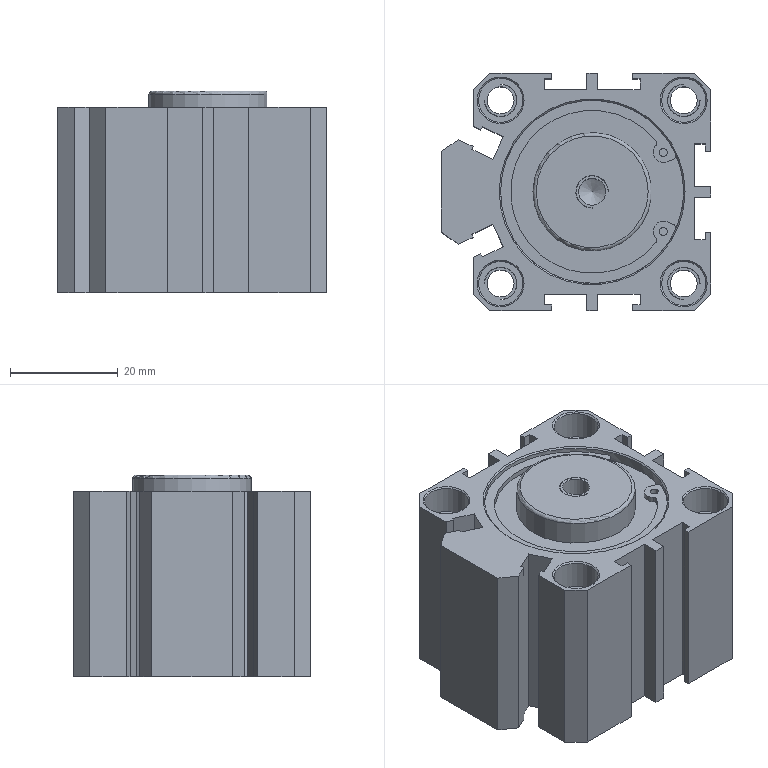Part | STEP file | Tube necking machine_id250_x_t | 1 solid | 212 faces | box 50 x 44 x 37.5 mm | volume 59062 mm3 | plane 138 | cylinder 39 | other 24 | cone 10 | torus 1 | commonest cylinder face diameters 8.2 x8 1.5 x6 5 x5 5.95 x5 6.05 x5 2 x4